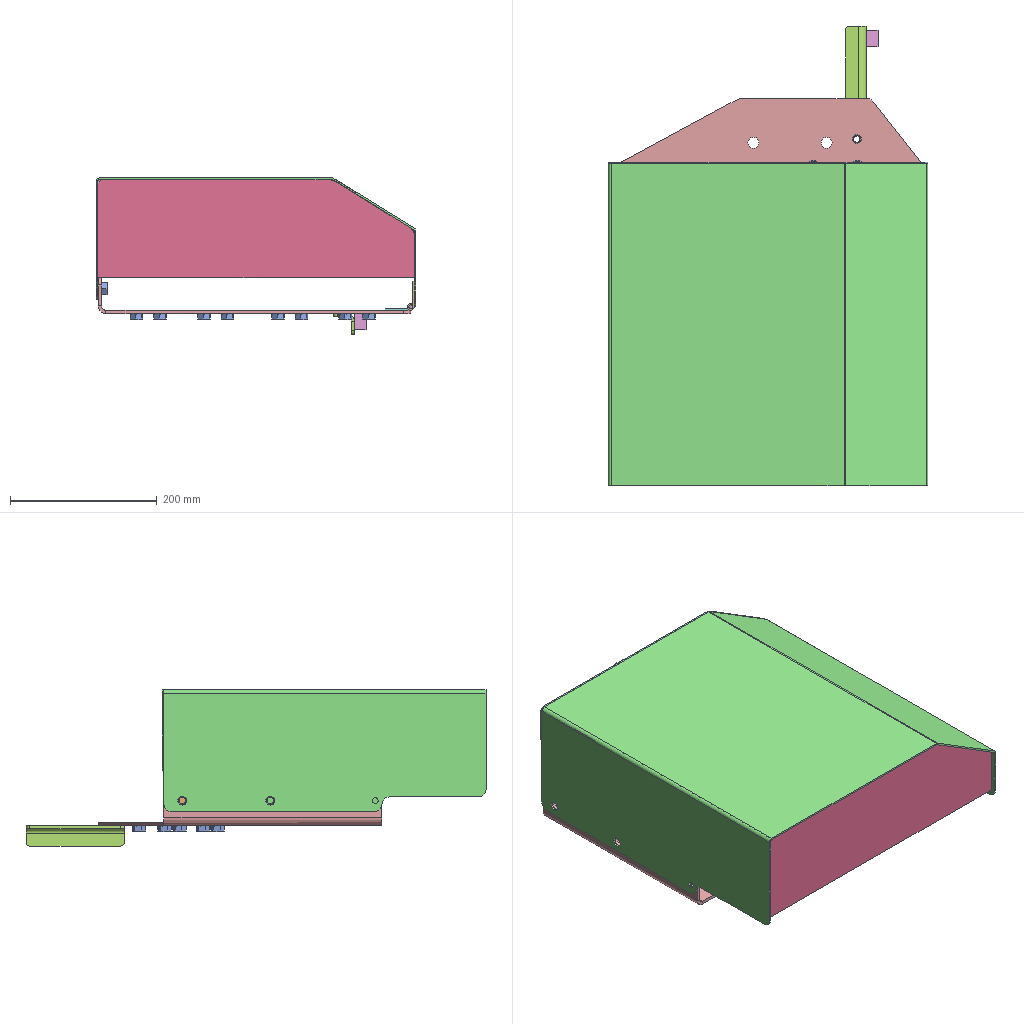Assembly | SolidWorks | 13 different items | 27 placed | box 436 x 627 x 213 mm
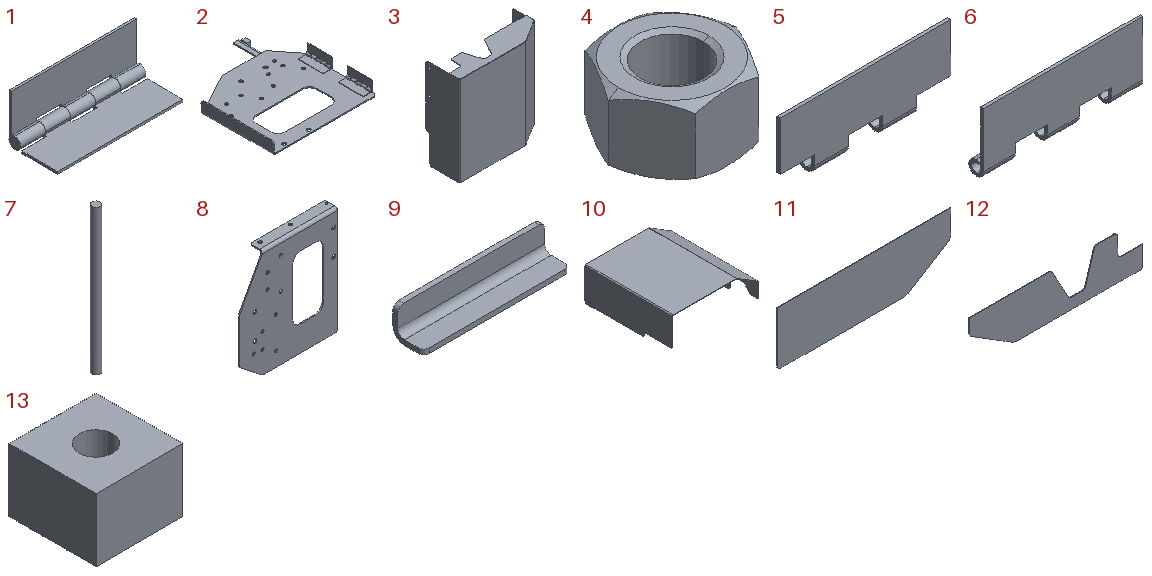Parts list (item | name | quantity | parent item | size | volume | features):
1 | (subassembly) | x2 | in 2 | 102 x 39.7 x 39.7 mm | 18759 mm3 | -
2 | (subassembly) | x1 | - | 430.7 x 485 x 77 mm | 689394 mm3 | features LocalLPattern 1, ReferencePattern 1
3 | (subassembly) | x1 | - | 436 x 176 x 441.3 mm | 908133 mm3 | -
4 | - | x11 | in 2 | 27.713 x 24 x 14.8 mm | 5071 mm3 | features RevCut 2, Chamfer 1, Extrusion 1, LPattern 1
5 | - | x2 | in 1 | 102 x 9.4 x 39.7 mm | 7631 mm3 | features FlatPattern 1, ICE 1, SMBaseFlange 1, SheetMetal 1
6 | - | x2 | in 1 | 102 x 9.4 x 39.7 mm | 8617 mm3 | features FlatPattern 1, ICE 1, SMBaseFlange 1, SheetMetal 1
7 | - | x2 | in 1 | 5.6 x 5.6 x 102 mm | 2512 mm3 | features Extrusion 1
8 | - | x1 | in 2 | 386 x 49 x 426 mm | 601864 mm3 | features ICE 2, Fillet 1, FlatPattern 1, SMBaseFlange 1, SheetMetal 1
9 | - | x1 | in 2 | 134 x 28 x 28 mm | 28823 mm3 | features Fillet 1, FlatPattern 1, SMBaseFlange 1, SheetMetal 1
10 | - | x1 | in 3 | 436 x 439 x 176 mm | 705533 mm3 | features ICE 2, Fillet 1, FlatPattern 1, SMBaseFlange 1, SheetMetal 1
11 | - | x1 | in 3 | 431.35 x 2.3 x 134 mm | 124034 mm3 | features Chamfer 2, FlatPattern 1, SMBaseFlange 1, SheetMetal 1
12 | - | x1 | in 3 | 436 x 2.3 x 110 mm | 78566 mm3 | features Chamfer 2, Fillet 1, FlatPattern 1, SMBaseFlange 1, SheetMetal 1
13 | - | x1 | in 2 | 22 x 22 x 16 mm | 6836 mm3 | features Extrusion 1, HoleWzd 1
Mates (type | each side: item.copy, entity, surface, feature):
In the top assembly
Coincident | 6.1 face plane Base-Flange1 | 10.1 face plane Base-Flange1
Concentric | 8.1 face cylinder Cut-Extrude2 | 10.1 face cylinder Cut-Extrude1 | 2 times
In subassembly 3
DistanceDim | 11.1 face plane Base-Flange1 | 10.2 face plane Base-Flange1
Coincident | 10.2 face plane Base-Flange1 | 11.1 face plane Base-Flange1 | 2 times
Coincident | 10.2 face plane Base-Flange1 | 12.1 face plane Base-Flange1 | 3 times
In subassembly 2
Concentric | 8.2 face cylinder Cut-Extrude2 | 4.1 face cone EndChamfer
Coincident | 8.2 face plane Base-Flange1 | 4.1 face plane BaseNut
Concentric | 8.2 face cylinder Cut-Extrude2 | 4.2 face cone EndChamfer
Coincident | 8.2 face plane Base-Flange1 | 4.2 face plane BaseNut
Parallel | 8.2 face plane Base-Flange1 | 4.2 face plane BaseNut
Coincident | 4.1 face plane BaseNut | 4.2 face plane BaseNut
Concentric | 8.2 face cylinder Cut-Extrude1 | 4.3 face cone EndChamfer
Coincident | 8.2 face plane Base-Flange1 | 4.3 face plane BaseNut
Concentric | 8.2 face cylinder Cut-Extrude1 | 4.4 face cone EndChamfer
Coincident | 8.2 face plane Base-Flange1 | 4.4 face plane BaseNut
Concentric | 8.2 face cylinder Cut-Extrude1 | 4.5 face cone EndChamfer
Coincident | 8.2 face plane Base-Flange1 | 4.5 face plane BaseNut
Concentric | 8.2 face cylinder Cut-Extrude1 | 4.6 face cone EndChamfer
Coincident | 8.2 face plane Base-Flange1 | 4.6 face plane BaseNut
Concentric | 8.2 face cylinder Cut-Extrude1 | 4.7 face cone EndChamfer
Coincident | 8.2 face plane Base-Flange1 | 4.7 face plane BaseNut
Concentric | 8.2 face cylinder Cut-Extrude1 | 4.8 face cone EndChamfer
Coincident | 8.2 face plane Base-Flange1 | 4.8 face plane BaseNut
Concentric | 8.2 face cylinder Cut-Extrude1 | 4.9 face cone EndChamfer
Coincident | 8.2 face plane Base-Flange1 | 4.9 face plane BaseNut
Concentric | 8.2 face cylinder Cut-Extrude1 | 4.10 face cone EndChamfer
Coincident | 8.2 face plane Base-Flange1 | 4.10 face plane BaseNut
Concentric | 8.2 face cylinder Cut-Extrude1 | 4.11 face cone EndChamfer
Coincident | 8.2 face plane Base-Flange1 | 4.11 face plane BaseNut
Coincident | 8.2 face plane Base-Flange1 | 9.1 face plane Base-Flange1
DistanceDim | 8.2 face cylinder Cut-Extrude1 | 9.1 face plane Base-Flange1
DistanceDim | 9.1 face plane Base-Flange1 | 8.2 face cylinder Cut-Extrude1
Parallel | 8.2 face plane Base-Flange1 | 9.1 face plane Base-Flange1
Coincident | 9.1 face plane Base-Flange1 | 13.1 face plane Boss-Extrude1 | 2 times
DistanceDim | 13.1 face cylinder M10 Tapped Hole1 | 9.1 face plane Base-Flange1
Coincident | 8.2 face plane Base-Flange1 | 5.1 face plane Base-Flange1
DistanceDim | 5.1 face plane Base-Flange1 | 8.2 face plane Base-Flange1 | 2 times
In subassembly 1
Concentric | 5.2 face cylinder Base Bend 1 | 6.2 face cylinder Base Bend 1
Coincident | 5.2 face plane Base-Flange1 | 6.2 face plane Base-Flange1
Perpendicular | 5.2 face plane Base-Flange1 | 6.2 face plane Base-Flange1
InPlace | 6.2 face plane Base-Flange1 | 7.1 plane